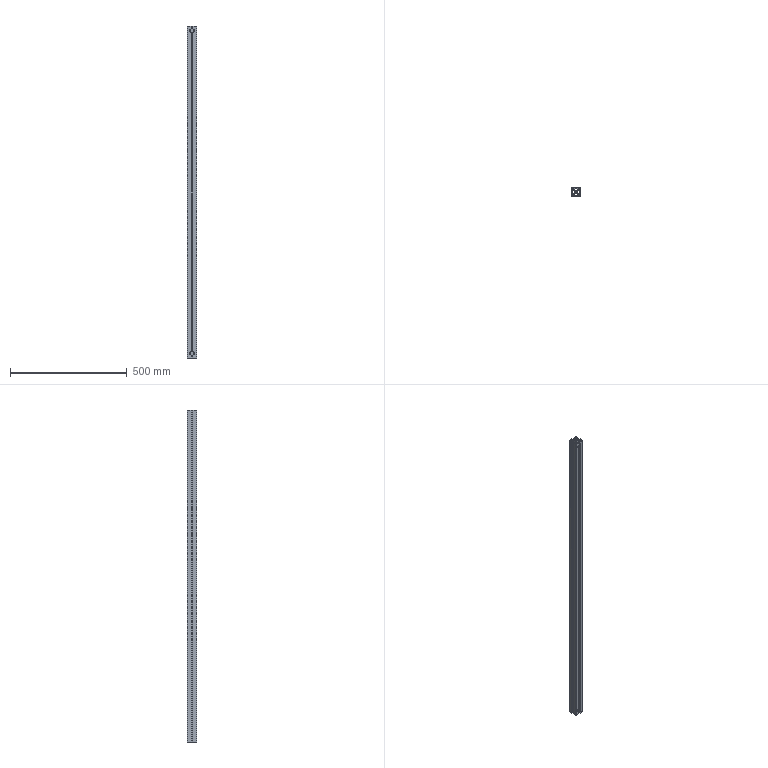Part | STEP file | 09-04 aluminium profile 4040-1420 | 1 solid | 93 faces | box 40 x 40 x 1420 mm | volume 998834 mm3 | plane 62 | cylinder 31 | commonest cylinder face diameters 19 x9 8 x8 18.5 x8 2 x4 6.8 x2